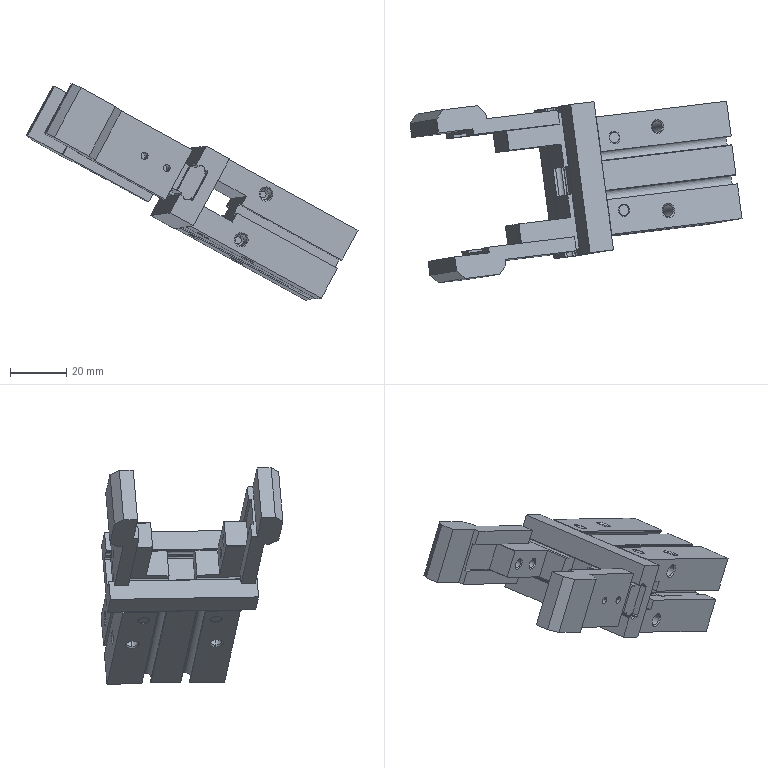Part | SolidWorks | 5 solids | 291 faces | box 117.707 x 64.465 x 76.746 mm | volume 74961 mm3 | plane 152 | cylinder 77 | cone 62 | commonest cylinder face diameters 4.134 x20 2.5 x17 0.4 x8 3.242 x8 5.02 x8 4.2 x6